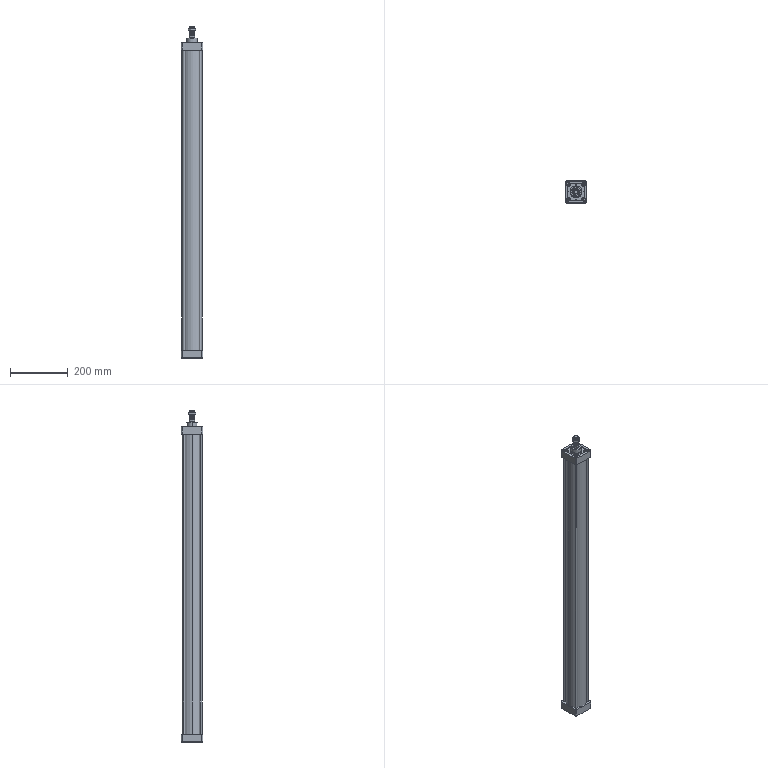Part | SolidWorks | 3 solids | 426 faces | box 75 x 75 x 1153 mm | volume 1669537 mm3 | plane 185 | cylinder 149 | cone 58 | torus 26 | spline 8 | commonest cylinder face diameters 16 x31 15.806 x30 11.6 x16 12 x16 2 x10 6 x8